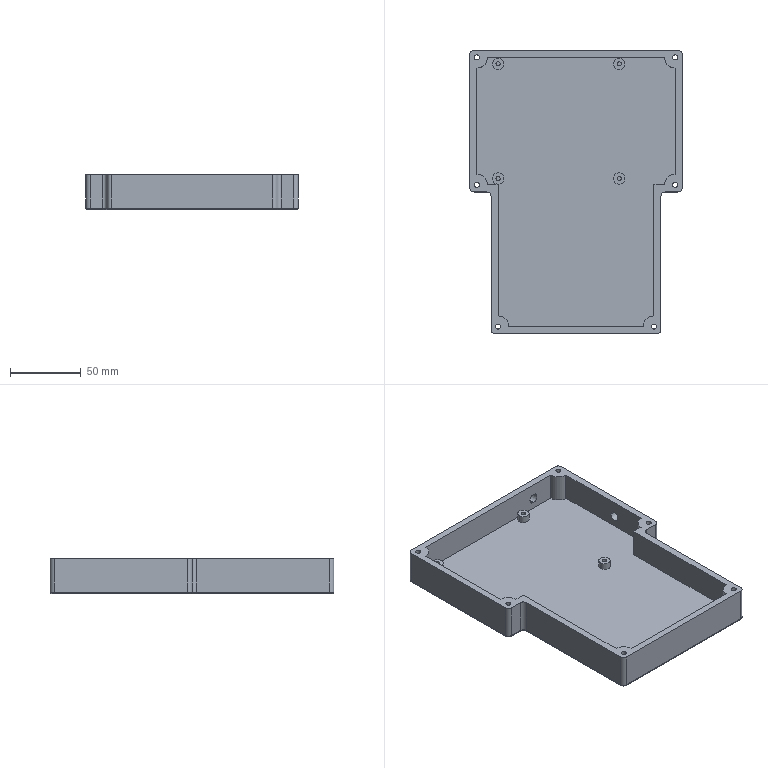Part | SolidWorks | features ICE 7, Fillet 2, Extrusion 1 | 1 solid | 107 faces | box 150 x 200 x 25 mm | volume 205338 mm3 | cylinder 66 | plane 33 | torus 8 | commonest cylinder face diameters 3.5 x12 7.5 x12 2 x8 3 x8 6 x8 8 x8